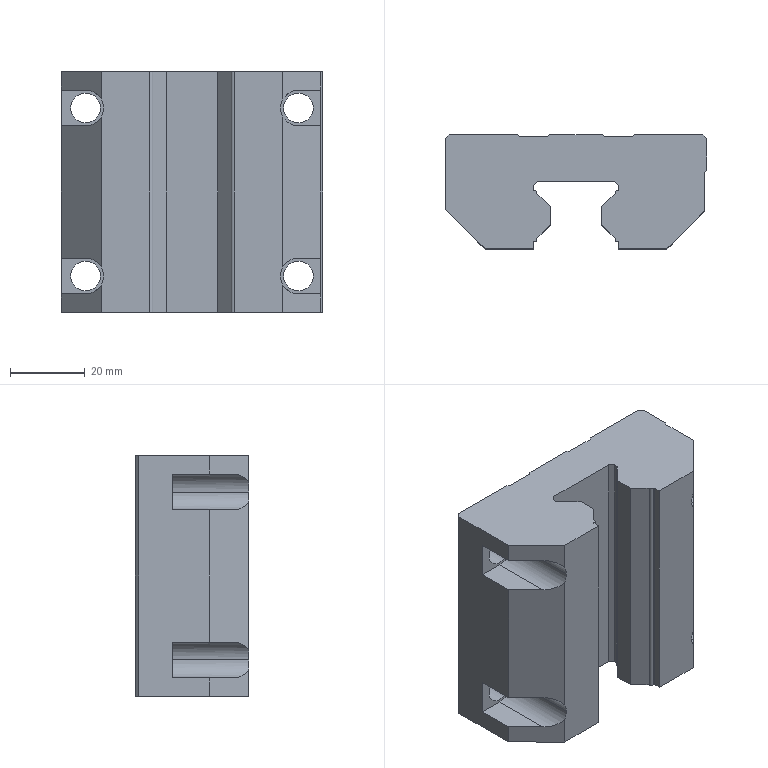Part | STEP file | 2026.6.15-Main Assembly图.sldasm-Part-17 | 1 solid | 291 faces | box 70 x 30.5 x 64.5 mm | volume 99534 mm3 | plane 162 | spline 93 | cylinder 32 | cone 4 | commonest cylinder face diameters 8 x12 1.629 x8 9.6 x8 6.4 x4